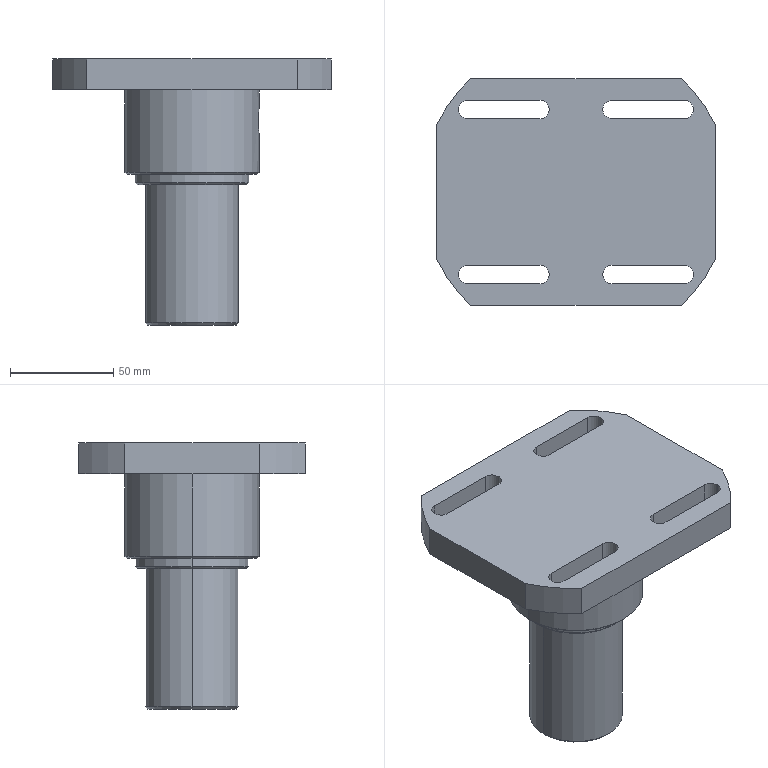Part | STEP file | LM-05-1162 modified_default | 1 solid | 55 faces | box 135 x 110 x 129 mm | volume 443950 mm3 | cylinder 26 | plane 17 | cone 12 | commonest cylinder face diameters 9 x12 150 x4 6.8 x2 10.2 x2 45 x2 55 x2